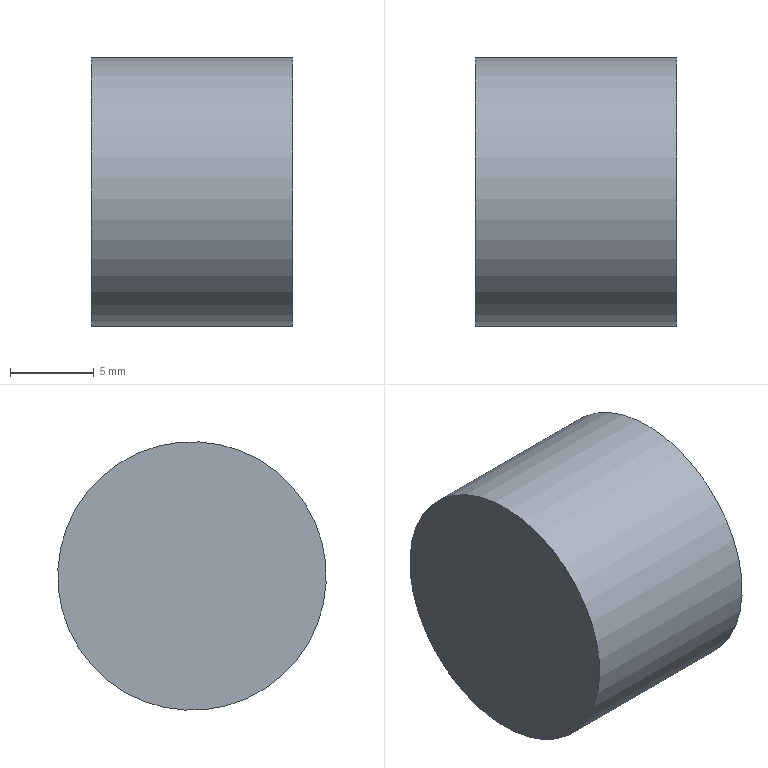Part | NX | features solid 2 | 1 solid | 10 faces | box 12 x 16 x 16 mm | volume 2025 mm3 | plane 9 | cylinder 1 | commonest cylinder face diameters 16 x1
STEP:
#1=CARTESIAN_POINT('',(212.,913.163,-221.52));
#2=VERTEX_POINT('',#1);
#3=CARTESIAN_POINT('',(212.,915.233,-213.793));
#4=DIRECTION('',(-1.,0.000000001,-0.000000005));
#5=DIRECTION('',(0.000000004,-0.2588,-0.9659));
#6=AXIS2_PLACEMENT_3D('',#3,#4,#5);
#7=CIRCLE('',#6,8.);
#8=EDGE_CURVE('',#2,#2,#7,.T.);
#9=ORIENTED_EDGE('',*,*,#8,.F.);
#10=EDGE_LOOP('',(#9));
#11=FACE_BOUND('',#10,.T.);
#12=CARTESIAN_POINT('',(224.,913.163,-221.52));
#13=VERTEX_POINT('',#12);
#14=CARTESIAN_POINT('',(224.,915.233,-213.793));
#15=DIRECTION('',(-1.,0.000000001,-0.000000005));
#16=DIRECTION('',(0.000000004,-0.2588,-0.9659));
#17=AXIS2_PLACEMENT_3D('',#14,#15,#16);
#18=CIRCLE('',#17,8.);
#19=EDGE_CURVE('',#13,#13,#18,.T.);
#20=ORIENTED_EDGE('',*,*,#19,.T.);
#21=EDGE_LOOP('',(#20));
#22=FACE_BOUND('',#21,.T.);
#23=CARTESIAN_POINT('',(212.,915.233,-213.793));
#24=DIRECTION('',(1.,-0.000000001,0.000000005));
#25=DIRECTION('',(0.000000004,-0.2588,-0.9659));
#26=AXIS2_PLACEMENT_3D('',#23,#24,#25);
#27=CYLINDRICAL_SURFACE('',#26,8.);
#28=ADVANCED_FACE('',(#11,#22),#27,.T.);
#29=ORIENTED_EDGE('',*,*,#8,.T.);
#30=EDGE_LOOP('',(#29));
#31=FACE_BOUND('',#30,.T.);
#32=CARTESIAN_POINT('',(212.,915.233,-213.793));
#33=DIRECTION('',(1.,-0.000000001,0.000000005));
#34=DIRECTION('',(0.000000004,-0.2588,-0.9659));
#35=AXIS2_PLACEMENT_3D('',#32,#33,#34);
#36=PLANE('',#35);
#37=ADVANCED_FACE('',(#31),#36,.F.);
#38=CARTESIAN_POINT('',(224.,919.695,-214.988));
#39=VERTEX_POINT('',#38);
#40=CARTESIAN_POINT('',(224.,916.429,-218.254));
#41=VERTEX_POINT('',#40);
#42=CARTESIAN_POINT('',(224.,919.695,-214.988));
#43=DIRECTION('',(0.000000003,-0.7071,-0.7071));
#44=VECTOR('',#43,1000.);
#45=LINE('',#42,#44);
#46=EDGE_CURVE('',#39,#41,#45,.T.);
#47=ORIENTED_EDGE('',*,*,#46,.T.);
#48=CARTESIAN_POINT('',(224.,911.967,-217.059));
#49=VERTEX_POINT('',#48);
#50=CARTESIAN_POINT('',(224.,911.967,-217.059));
#51=DIRECTION('',(0.000000003,0.9659,-0.2588));
#52=VECTOR('',#51,1000.);
#53=LINE('',#50,#52);
#54=EDGE_CURVE('',#49,#41,#53,.T.);
#55=ORIENTED_EDGE('',*,*,#54,.F.);
#56=CARTESIAN_POINT('',(224.,910.772,-212.597));
#57=VERTEX_POINT('',#56);
#58=CARTESIAN_POINT('',(224.,910.772,-212.597));
#59=DIRECTION('',(0.000000005,0.2588,-0.9659));
#60=VECTOR('',#59,1000.);
#61=LINE('',#58,#60);
#62=EDGE_CURVE('',#57,#49,#61,.T.);
#63=ORIENTED_EDGE('',*,*,#62,.F.);
#64=CARTESIAN_POINT('',(224.,914.038,-209.331));
#65=VERTEX_POINT('',#64);
#66=CARTESIAN_POINT('',(224.,914.038,-209.331));
#67=DIRECTION('',(0.000000003,-0.7071,-0.7071));
#68=VECTOR('',#67,1000.);
#69=LINE('',#66,#68);
#70=EDGE_CURVE('',#65,#57,#69,.T.);
#71=ORIENTED_EDGE('',*,*,#70,.F.);
#72=CARTESIAN_POINT('',(224.,918.499,-210.527));
#73=VERTEX_POINT('',#72);
#74=CARTESIAN_POINT('',(224.,914.038,-209.331));
#75=DIRECTION('',(0.000000003,0.9659,-0.2588));
#76=VECTOR('',#75,1000.);
#77=LINE('',#74,#76);
#78=EDGE_CURVE('',#65,#73,#77,.T.);
#79=ORIENTED_EDGE('',*,*,#78,.T.);
#80=CARTESIAN_POINT('',(224.,918.499,-210.527));
#81=DIRECTION('',(0.000000005,0.2588,-0.9659));
#82=VECTOR('',#81,1000.);
#83=LINE('',#80,#82);
#84=EDGE_CURVE('',#73,#39,#83,.T.);
#85=ORIENTED_EDGE('',*,*,#84,.T.);
#86=EDGE_LOOP('',(#47,#55,#63,#71,#79,#85));
#87=FACE_BOUND('',#86,.T.);
#88=ORIENTED_EDGE('',*,*,#19,.F.);
#89=EDGE_LOOP('',(#88));
#90=FACE_BOUND('',#89,.T.);
#91=CARTESIAN_POINT('',(224.,915.233,-213.793));
#92=DIRECTION('',(1.,-0.000000001,0.000000005));
#93=DIRECTION('',(0.000000004,-0.2588,-0.9659));
#94=AXIS2_PLACEMENT_3D('',#91,#92,#93);
#95=PLANE('',#94);
#96=ADVANCED_FACE('',(#87,#90),#95,.T.);
#97=ORIENTED_EDGE('',*,*,#46,.F.);
#98=CARTESIAN_POINT('',(217.,919.695,-214.988));
#99=VERTEX_POINT('',#98);
#100=CARTESIAN_POINT('',(217.,919.695,-214.988));
#101=DIRECTION('',(1.,-0.000000001,0.000000005));
#102=VECTOR('',#101,1000.);
#103=LINE('',#100,#102);
#104=EDGE_CURVE('',#99,#39,#103,.T.);
#105=ORIENTED_EDGE('',*,*,#104,.F.);
#106=CARTESIAN_POINT('',(217.,916.429,-218.254));
#107=VERTEX_POINT('',#106);
#108=CARTESIAN_POINT('',(217.,919.695,-214.988));
#109=DIRECTION('',(0.000000003,-0.7071,-0.7071));
#110=VECTOR('',#109,1000.);
#111=LINE('',#108,#110);
#112=EDGE_CURVE('',#99,#107,#111,.T.);
#113=ORIENTED_EDGE('',*,*,#112,.T.);
#114=CARTESIAN_POINT('',(217.,916.429,-218.254));
#115=DIRECTION('',(1.,-0.000000001,0.000000005));
#116=VECTOR('',#115,1000.);
#117=LINE('',#114,#116);
#118=EDGE_CURVE('',#107,#41,#117,.T.);
#119=ORIENTED_EDGE('',*,*,#118,.T.);
#120=EDGE_LOOP('',(#97,#105,#113,#119));
#121=FACE_BOUND('',#120,.T.);
#122=CARTESIAN_POINT('',(217.,919.695,-214.988));
#123=DIRECTION('',(0.000000004,0.7071,-0.7071));
#124=DIRECTION('',(0.,-0.7071,-0.7071));
#125=AXIS2_PLACEMENT_3D('',#122,#123,#124);
#126=PLANE('',#125);
#127=ADVANCED_FACE('',(#121),#126,.F.);
#128=ORIENTED_EDGE('',*,*,#54,.T.);
#129=ORIENTED_EDGE('',*,*,#118,.F.);
#130=CARTESIAN_POINT('',(217.,911.967,-217.059));
#131=VERTEX_POINT('',#130);
#132=CARTESIAN_POINT('',(217.,911.967,-217.059));
#133=DIRECTION('',(0.000000003,0.9659,-0.2588));
#134=VECTOR('',#133,1000.);
#135=LINE('',#132,#134);
#136=EDGE_CURVE('',#131,#107,#135,.T.);
#137=ORIENTED_EDGE('',*,*,#136,.F.);
#138=CARTESIAN_POINT('',(217.,911.967,-217.059));
#139=DIRECTION('',(1.,-0.000000001,0.000000005));
#140=VECTOR('',#139,1000.);
#141=LINE('',#138,#140);
#142=EDGE_CURVE('',#131,#49,#141,.T.);
#143=ORIENTED_EDGE('',*,*,#142,.T.);
#144=EDGE_LOOP('',(#128,#129,#137,#143));
#145=FACE_BOUND('',#144,.T.);
#146=CARTESIAN_POINT('',(217.,911.967,-217.059));
#147=DIRECTION('',(-0.000000004,0.2588,0.9659));
#148=DIRECTION('',(0.,0.9659,-0.2588));
#149=AXIS2_PLACEMENT_3D('',#146,#147,#148);
#150=PLANE('',#149);
#151=ADVANCED_FACE('',(#145),#150,.T.);
#152=ORIENTED_EDGE('',*,*,#62,.T.);
#153=ORIENTED_EDGE('',*,*,#142,.F.);
#154=CARTESIAN_POINT('',(217.,910.772,-212.597));
#155=VERTEX_POINT('',#154);
#156=CARTESIAN_POINT('',(217.,910.772,-212.597));
#157=DIRECTION('',(0.000000005,0.2588,-0.9659));
#158=VECTOR('',#157,1000.);
#159=LINE('',#156,#158);
#160=EDGE_CURVE('',#155,#131,#159,.T.);
#161=ORIENTED_EDGE('',*,*,#160,.F.);
#162=CARTESIAN_POINT('',(217.,910.772,-212.597));
#163=DIRECTION('',(1.,-0.000000001,0.000000005));
#164=VECTOR('',#163,1000.);
#165=LINE('',#162,#164);
#166=EDGE_CURVE('',#155,#57,#165,.T.);
#167=ORIENTED_EDGE('',*,*,#166,.T.);
#168=EDGE_LOOP('',(#152,#153,#161,#167));
#169=FACE_BOUND('',#168,.T.);
#170=CARTESIAN_POINT('',(217.,910.772,-212.597));
#171=DIRECTION('',(0.,0.9659,0.2588));
#172=DIRECTION('',(0.,0.2588,-0.9659));
#173=AXIS2_PLACEMENT_3D('',#170,#171,#172);
#174=PLANE('',#173);
#175=ADVANCED_FACE('',(#169),#174,.T.);
#176=ORIENTED_EDGE('',*,*,#70,.T.);
#177=ORIENTED_EDGE('',*,*,#166,.F.);
#178=CARTESIAN_POINT('',(217.,914.038,-209.331));
#179=VERTEX_POINT('',#178);
#180=CARTESIAN_POINT('',(217.,914.038,-209.331));
#181=DIRECTION('',(0.000000003,-0.7071,-0.7071));
#182=VECTOR('',#181,1000.);
#183=LINE('',#180,#182);
#184=EDGE_CURVE('',#179,#155,#183,.T.);
#185=ORIENTED_EDGE('',*,*,#184,.F.);
#186=CARTESIAN_POINT('',(217.,914.038,-209.331));
#187=DIRECTION('',(1.,-0.000000001,0.000000005));
#188=VECTOR('',#187,1000.);
#189=LINE('',#186,#188);
#190=EDGE_CURVE('',#179,#65,#189,.T.);
#191=ORIENTED_EDGE('',*,*,#190,.T.);
#192=EDGE_LOOP('',(#176,#177,#185,#191));
#193=FACE_BOUND('',#192,.T.);
#194=CARTESIAN_POINT('',(217.,914.038,-209.331));
#195=DIRECTION('',(0.000000004,0.7071,-0.7071));
#196=DIRECTION('',(0.,-0.7071,-0.7071));
#197=AXIS2_PLACEMENT_3D('',#194,#195,#196);
#198=PLANE('',#197);
#199=ADVANCED_FACE('',(#193),#198,.T.);
#200=ORIENTED_EDGE('',*,*,#78,.F.);
#201=ORIENTED_EDGE('',*,*,#190,.F.);
#202=CARTESIAN_POINT('',(217.,918.499,-210.527));
#203=VERTEX_POINT('',#202);
#204=CARTESIAN_POINT('',(217.,914.038,-209.331));
#205=DIRECTION('',(0.000000003,0.9659,-0.2588));
#206=VECTOR('',#205,1000.);
#207=LINE('',#204,#206);
#208=EDGE_CURVE('',#179,#203,#207,.T.);
#209=ORIENTED_EDGE('',*,*,#208,.T.);
#210=CARTESIAN_POINT('',(217.,918.499,-210.527));
#211=DIRECTION('',(1.,-0.000000001,0.000000005));
#212=VECTOR('',#211,1000.);
#213=LINE('',#210,#212);
#214=EDGE_CURVE('',#203,#73,#213,.T.);
#215=ORIENTED_EDGE('',*,*,#214,.T.);
#216=EDGE_LOOP('',(#200,#201,#209,#215));
#217=FACE_BOUND('',#216,.T.);
#218=CARTESIAN_POINT('',(217.,914.038,-209.331));
#219=DIRECTION('',(-0.000000004,0.2588,0.9659));
#220=DIRECTION('',(1.,0.000000001,0.000000004));
#221=AXIS2_PLACEMENT_3D('',#218,#219,#220);
#222=PLANE('',#221);
#223=ADVANCED_FACE('',(#217),#222,.F.);
#224=ORIENTED_EDGE('',*,*,#84,.F.);
#225=ORIENTED_EDGE('',*,*,#214,.F.);
#226=CARTESIAN_POINT('',(217.,918.499,-210.527));
#227=DIRECTION('',(0.000000005,0.2588,-0.9659));
#228=VECTOR('',#227,1000.);
#229=LINE('',#226,#228);
#230=EDGE_CURVE('',#203,#99,#229,.T.);
#231=ORIENTED_EDGE('',*,*,#230,.T.);
#232=ORIENTED_EDGE('',*,*,#104,.T.);
#233=EDGE_LOOP('',(#224,#225,#231,#232));
#234=FACE_BOUND('',#233,.T.);
#235=CARTESIAN_POINT('',(217.,918.499,-210.527));
#236=DIRECTION('',(0.,0.9659,0.2588));
#237=DIRECTION('',(0.,0.2588,-0.9659));
#238=AXIS2_PLACEMENT_3D('',#235,#236,#237);
#239=PLANE('',#238);
#240=ADVANCED_FACE('',(#234),#239,.F.);
#241=ORIENTED_EDGE('',*,*,#112,.F.);
#242=ORIENTED_EDGE('',*,*,#230,.F.);
#243=ORIENTED_EDGE('',*,*,#208,.F.);
#244=ORIENTED_EDGE('',*,*,#184,.T.);
#245=ORIENTED_EDGE('',*,*,#160,.T.);
#246=ORIENTED_EDGE('',*,*,#136,.T.);
#247=EDGE_LOOP('',(#241,#242,#243,#244,#245,#246));
#248=FACE_BOUND('',#247,.T.);
#249=CARTESIAN_POINT('',(217.,913.163,-221.52));
#250=DIRECTION('',(-1.,0.000000001,-0.000000005));
#251=DIRECTION('',(-0.000000004,0.2588,0.9659));
#252=AXIS2_PLACEMENT_3D('',#249,#250,#251);
#253=PLANE('',#252);
#254=ADVANCED_FACE('',(#248),#253,.F.);
#255=CLOSED_SHELL('',(#28,#37,#96,#127,#151,#175,#199,#223,#240,#254));
#256=MANIFOLD_SOLID_BREP('',#255);
#257=(LENGTH_UNIT()NAMED_UNIT(*)SI_UNIT(.MILLI.,.METRE.));
#258=UNCERTAINTY_MEASURE_WITH_UNIT(LENGTH_MEASURE(0.00001),#257,'','');
#259=(NAMED_UNIT(*)PLANE_ANGLE_UNIT()SI_UNIT($,.RADIAN.));
#260=(NAMED_UNIT(*)SI_UNIT($,.STERADIAN.)SOLID_ANGLE_UNIT());
#261=(GEOMETRIC_REPRESENTATION_CONTEXT(3)GLOBAL_UNCERTAINTY_ASSIGNED_CONTEXT((#258))GLOBAL_UNIT_ASSIGNED_CONTEXT((#257,#259,#260))REPRESENTATION_CONTEXT('',''));
#262=ADVANCED_BREP_SHAPE_REPRESENTATION('',(#256),#261);